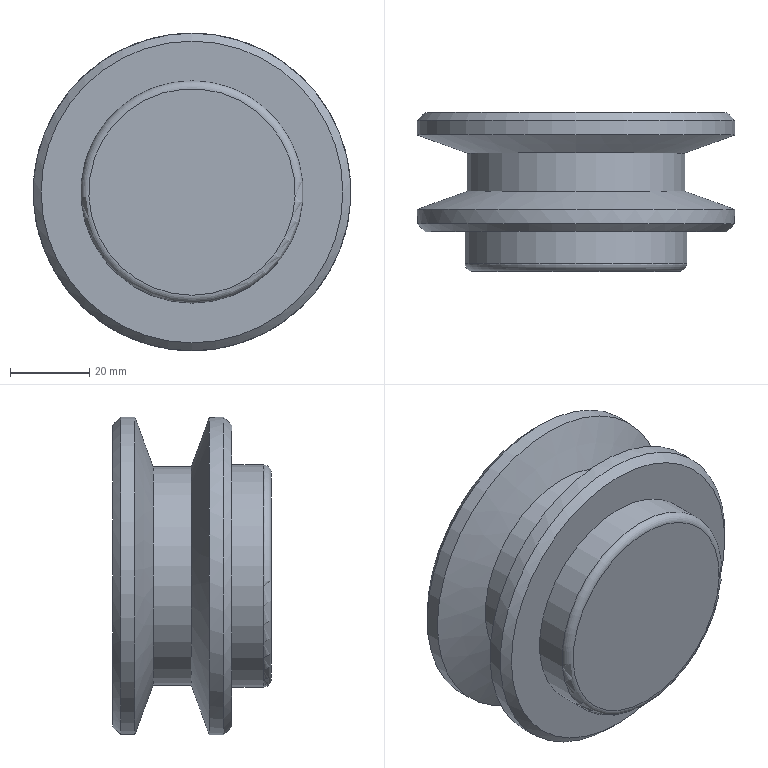Part | STEP file | Tube feed_id138_x_t | 1 solid | 12 faces | box 80 x 40 x 80 mm | volume 135943 mm3 | cylinder 4 | cone 4 | plane 3 | torus 1 | commonest cylinder face diameters 80 x2 55 x1 56 x1
STEP:
#1=CARTESIAN_POINT('',(0.,0.,0.));
#2=DIRECTION('',(0.,0.,1.));
#3=DIRECTION('',(1.,0.,0.));
#4=AXIS2_PLACEMENT_3D('',#1,#2,#3);
#5=CARTESIAN_POINT('',(-268.5,583.936,-125.5));
#6=VERTEX_POINT('',#5);
#7=CARTESIAN_POINT('',(-268.5,583.936,-205.5));
#8=VERTEX_POINT('',#7);
#9=CARTESIAN_POINT('',(-268.5,583.936,-165.5));
#10=DIRECTION('',(0.,1.,0.));
#11=DIRECTION('',(0.,0.,1.));
#12=AXIS2_PLACEMENT_3D('',#9,#10,#11);
#13=CIRCLE('',#12,40.);
#14=CARTESIAN_POINT('',(-268.5,601.936,-165.5));
#15=DIRECTION('',(0.,-1.,0.));
#16=DIRECTION('',(0.,0.,-1.));
#17=AXIS2_PLACEMENT_3D('',#14,#15,#16);
#18=CYLINDRICAL_SURFACE('',#17,40.);
#19=CARTESIAN_POINT('',(3.142,18.));
#20=DIRECTION('',(-1.,0.));
#21=VECTOR('',#20,1.);
#22=LINE('',#19,#21);
#23=(GEOMETRIC_REPRESENTATION_CONTEXT(2)PARAMETRIC_REPRESENTATION_CONTEXT()REPRESENTATION_CONTEXT('',''));
#24=DEFINITIONAL_REPRESENTATION('',(#22),#23);
#25=PCURVE('',#18,#24);
#26=CARTESIAN_POINT('',(-268.5,583.936,-165.5));
#27=DIRECTION('',(0.,1.,0.));
#28=DIRECTION('',(0.,0.,1.));
#29=AXIS2_PLACEMENT_3D('',#26,#27,#28);
#30=CONICAL_SURFACE('',#29,40.,0.7854);
#31=CARTESIAN_POINT('',(0.,0.));
#32=DIRECTION('',(1.,0.));
#33=VECTOR('',#32,1.);
#34=LINE('',#31,#33);
#35=(GEOMETRIC_REPRESENTATION_CONTEXT(2)PARAMETRIC_REPRESENTATION_CONTEXT()REPRESENTATION_CONTEXT('',''));
#36=DEFINITIONAL_REPRESENTATION('',(#34),#35);
#37=PCURVE('',#30,#36);
#38=SURFACE_CURVE('',#13,(#25,#37),.PCURVE_S1.);
#39=EDGE_CURVE('',#6,#8,#38,.T.);
#40=ORIENTED_EDGE('',*,*,#39,.T.);
#41=CARTESIAN_POINT('',(-268.5,587.568,-205.5));
#42=VERTEX_POINT('',#41);
#43=CARTESIAN_POINT('',(-268.5,587.568,-205.5));
#44=CARTESIAN_POINT('',(-268.5,583.936,-205.5));
#45=B_SPLINE_CURVE_WITH_KNOTS('',1,(#43,#44),.UNSPECIFIED.,.F.,.F.,(2,2),(14.368,18.),.PIECEWISE_BEZIER_KNOTS.);
#46=CARTESIAN_POINT('',(0.,0.));
#47=DIRECTION('',(0.,1.));
#48=VECTOR('',#47,1.);
#49=LINE('',#46,#48);
#50=(GEOMETRIC_REPRESENTATION_CONTEXT(2)PARAMETRIC_REPRESENTATION_CONTEXT()REPRESENTATION_CONTEXT('',''));
#51=DEFINITIONAL_REPRESENTATION('',(#49),#50);
#52=PCURVE('',#18,#51);
#53=CARTESIAN_POINT('',(6.283,0.));
#54=DIRECTION('',(0.,1.));
#55=VECTOR('',#54,1.);
#56=LINE('',#53,#55);
#57=(GEOMETRIC_REPRESENTATION_CONTEXT(2)PARAMETRIC_REPRESENTATION_CONTEXT()REPRESENTATION_CONTEXT('',''));
#58=DEFINITIONAL_REPRESENTATION('',(#56),#57);
#59=PCURVE('',#18,#58);
#60=SEAM_CURVE('',#45,(#52,#59),.PCURVE_S1.);
#61=EDGE_CURVE('',#42,#8,#60,.T.);
#62=ORIENTED_EDGE('',*,*,#61,.F.);
#63=CARTESIAN_POINT('',(-268.5,587.568,-165.5));
#64=DIRECTION('',(0.,1.,0.));
#65=DIRECTION('',(0.,0.,-1.));
#66=AXIS2_PLACEMENT_3D('',#63,#64,#65);
#67=CIRCLE('',#66,40.);
#68=CARTESIAN_POINT('',(6.283,14.368));
#69=DIRECTION('',(-1.,0.));
#70=VECTOR('',#69,1.);
#71=LINE('',#68,#70);
#72=(GEOMETRIC_REPRESENTATION_CONTEXT(2)PARAMETRIC_REPRESENTATION_CONTEXT()REPRESENTATION_CONTEXT('',''));
#73=DEFINITIONAL_REPRESENTATION('',(#71),#72);
#74=PCURVE('',#18,#73);
#75=CARTESIAN_POINT('',(-268.5,591.936,-165.5));
#76=DIRECTION('',(0.,-1.,0.));
#77=DIRECTION('',(0.,0.,-1.));
#78=AXIS2_PLACEMENT_3D('',#75,#76,#77);
#79=CONICAL_SURFACE('',#78,28.,1.222);
#80=CARTESIAN_POINT('',(6.283,4.368));
#81=DIRECTION('',(-1.,0.));
#82=VECTOR('',#81,1.);
#83=LINE('',#80,#82);
#84=(GEOMETRIC_REPRESENTATION_CONTEXT(2)PARAMETRIC_REPRESENTATION_CONTEXT()REPRESENTATION_CONTEXT('',''));
#85=DEFINITIONAL_REPRESENTATION('',(#83),#84);
#86=PCURVE('',#79,#85);
#87=SURFACE_CURVE('',#67,(#74,#86),.PCURVE_S1.);
#88=EDGE_CURVE('',#42,#42,#87,.T.);
#89=ORIENTED_EDGE('',*,*,#88,.F.);
#90=ORIENTED_EDGE('',*,*,#61,.T.);
#91=CARTESIAN_POINT('',(-268.5,583.936,-165.5));
#92=DIRECTION('',(0.,1.,0.));
#93=DIRECTION('',(0.,0.,1.));
#94=AXIS2_PLACEMENT_3D('',#91,#92,#93);
#95=CIRCLE('',#94,40.);
#96=CARTESIAN_POINT('',(9.425,18.));
#97=DIRECTION('',(-1.,0.));
#98=VECTOR('',#97,1.);
#99=LINE('',#96,#98);
#100=(GEOMETRIC_REPRESENTATION_CONTEXT(2)PARAMETRIC_REPRESENTATION_CONTEXT()REPRESENTATION_CONTEXT('',''));
#101=DEFINITIONAL_REPRESENTATION('',(#99),#100);
#102=PCURVE('',#18,#101);
#103=CARTESIAN_POINT('',(0.,0.));
#104=DIRECTION('',(1.,0.));
#105=VECTOR('',#104,1.);
#106=LINE('',#103,#105);
#107=(GEOMETRIC_REPRESENTATION_CONTEXT(2)PARAMETRIC_REPRESENTATION_CONTEXT()REPRESENTATION_CONTEXT('',''));
#108=DEFINITIONAL_REPRESENTATION('',(#106),#107);
#109=PCURVE('',#30,#108);
#110=SURFACE_CURVE('',#95,(#102,#109),.PCURVE_S1.);
#111=EDGE_CURVE('',#8,#6,#110,.T.);
#112=ORIENTED_EDGE('',*,*,#111,.T.);
#113=EDGE_LOOP('',(#40,#62,#89,#90,#112));
#114=FACE_BOUND('',#113,.T.);
#115=ADVANCED_FACE('',(#114),#18,.T.);
#116=CARTESIAN_POINT('',(-268.5,581.936,-193.5));
#117=VERTEX_POINT('',#116);
#118=CARTESIAN_POINT('',(-268.5,581.936,-165.5));
#119=DIRECTION('',(0.,-1.,0.));
#120=DIRECTION('',(0.,0.,-1.));
#121=AXIS2_PLACEMENT_3D('',#118,#119,#120);
#122=CIRCLE('',#121,28.);
#123=CARTESIAN_POINT('',(-268.5,581.936,-165.5));
#124=DIRECTION('',(0.,1.,0.));
#125=DIRECTION('',(0.,0.,1.));
#126=AXIS2_PLACEMENT_3D('',#123,#124,#125);
#127=PLANE('',#126);
#128=CARTESIAN_POINT('',(-28.,0.));
#129=CARTESIAN_POINT('',(-28.,48.497));
#130=CARTESIAN_POINT('',(14.,24.249));
#131=CARTESIAN_POINT('',(56.,0.));
#132=CARTESIAN_POINT('',(14.,-24.249));
#133=CARTESIAN_POINT('',(-28.,-48.497));
#134=CARTESIAN_POINT('',(-28.,0.));
#135=(BOUNDED_CURVE()B_SPLINE_CURVE(2,(#128,#129,#130,#131,#132,#133,#134),.UNSPECIFIED.,.T.,.F.)B_SPLINE_CURVE_WITH_KNOTS((1,2,2,2,2,1),(-2.094,0.,2.094,4.189,6.283,8.378),.UNSPECIFIED.)CURVE()GEOMETRIC_REPRESENTATION_ITEM()RATIONAL_B_SPLINE_CURVE((1.,0.5,1.,0.5,1.,0.5,1.))REPRESENTATION_ITEM(''));
#136=(GEOMETRIC_REPRESENTATION_CONTEXT(2)PARAMETRIC_REPRESENTATION_CONTEXT()REPRESENTATION_CONTEXT('',''));
#137=DEFINITIONAL_REPRESENTATION('',(#135),#136);
#138=PCURVE('',#127,#137);
#139=CARTESIAN_POINT('',(-268.5,571.936,-165.5));
#140=DIRECTION('',(0.,1.,0.));
#141=DIRECTION('',(0.,0.,1.));
#142=AXIS2_PLACEMENT_3D('',#139,#140,#141);
#143=CYLINDRICAL_SURFACE('',#142,28.);
#144=CARTESIAN_POINT('',(9.425,10.));
#145=DIRECTION('',(-1.,0.));
#146=VECTOR('',#145,1.);
#147=LINE('',#144,#146);
#148=(GEOMETRIC_REPRESENTATION_CONTEXT(2)PARAMETRIC_REPRESENTATION_CONTEXT()REPRESENTATION_CONTEXT('',''));
#149=DEFINITIONAL_REPRESENTATION('',(#147),#148);
#150=PCURVE('',#143,#149);
#151=SURFACE_CURVE('',#122,(#138,#150),.PCURVE_S1.);
#152=EDGE_CURVE('',#117,#117,#151,.T.);
#153=ORIENTED_EDGE('',*,*,#152,.F.);
#154=EDGE_LOOP('',(#153));
#155=FACE_BOUND('',#154,.T.);
#156=CARTESIAN_POINT('',(-268.5,581.936,-127.5));
#157=VERTEX_POINT('',#156);
#158=CARTESIAN_POINT('',(-268.5,581.936,-165.5));
#159=DIRECTION('',(0.,-1.,0.));
#160=DIRECTION('',(0.,0.,1.));
#161=AXIS2_PLACEMENT_3D('',#158,#159,#160);
#162=CIRCLE('',#161,38.);
#163=CARTESIAN_POINT('',(38.,0.));
#164=CARTESIAN_POINT('',(38.,-65.818));
#165=CARTESIAN_POINT('',(-19.,-32.909));
#166=CARTESIAN_POINT('',(-76.,0.));
#167=CARTESIAN_POINT('',(-19.,32.909));
#168=CARTESIAN_POINT('',(38.,65.818));
#169=CARTESIAN_POINT('',(38.,0.));
#170=(BOUNDED_CURVE()B_SPLINE_CURVE(2,(#163,#164,#165,#166,#167,#168,#169),.UNSPECIFIED.,.T.,.F.)B_SPLINE_CURVE_WITH_KNOTS((1,2,2,2,2,1),(-2.094,0.,2.094,4.189,6.283,8.378),.UNSPECIFIED.)CURVE()GEOMETRIC_REPRESENTATION_ITEM()RATIONAL_B_SPLINE_CURVE((1.,0.5,1.,0.5,1.,0.5,1.))REPRESENTATION_ITEM(''));
#171=(GEOMETRIC_REPRESENTATION_CONTEXT(2)PARAMETRIC_REPRESENTATION_CONTEXT()REPRESENTATION_CONTEXT('',''));
#172=DEFINITIONAL_REPRESENTATION('',(#170),#171);
#173=PCURVE('',#127,#172);
#174=CARTESIAN_POINT('',(6.283,-2.));
#175=DIRECTION('',(-1.,0.));
#176=VECTOR('',#175,1.);
#177=LINE('',#174,#176);
#178=(GEOMETRIC_REPRESENTATION_CONTEXT(2)PARAMETRIC_REPRESENTATION_CONTEXT()REPRESENTATION_CONTEXT('',''));
#179=DEFINITIONAL_REPRESENTATION('',(#177),#178);
#180=PCURVE('',#30,#179);
#181=SURFACE_CURVE('',#162,(#173,#180),.PCURVE_S1.);
#182=EDGE_CURVE('',#157,#157,#181,.T.);
#183=ORIENTED_EDGE('',*,*,#182,.T.);
#184=EDGE_LOOP('',(#183));
#185=FACE_BOUND('',#184,.T.);
#186=ADVANCED_FACE('',(#155,#185),#127,.F.);
#187=ORIENTED_EDGE('',*,*,#182,.F.);
#188=CARTESIAN_POINT('',(-268.5,581.936,-127.5));
#189=CARTESIAN_POINT('',(-268.5,583.936,-125.5));
#190=B_SPLINE_CURVE_WITH_KNOTS('',1,(#188,#189),.UNSPECIFIED.,.F.,.F.,(2,2),(-2.828,0.),.PIECEWISE_BEZIER_KNOTS.);
#191=CARTESIAN_POINT('',(6.283,0.));
#192=DIRECTION('',(0.,1.));
#193=VECTOR('',#192,1.);
#194=LINE('',#191,#193);
#195=(GEOMETRIC_REPRESENTATION_CONTEXT(2)PARAMETRIC_REPRESENTATION_CONTEXT()REPRESENTATION_CONTEXT('',''));
#196=DEFINITIONAL_REPRESENTATION('',(#194),#195);
#197=PCURVE('',#30,#196);
#198=CARTESIAN_POINT('',(0.,0.));
#199=DIRECTION('',(0.,1.));
#200=VECTOR('',#199,1.);
#201=LINE('',#198,#200);
#202=(GEOMETRIC_REPRESENTATION_CONTEXT(2)PARAMETRIC_REPRESENTATION_CONTEXT()REPRESENTATION_CONTEXT('',''));
#203=DEFINITIONAL_REPRESENTATION('',(#201),#202);
#204=PCURVE('',#30,#203);
#205=SEAM_CURVE('',#190,(#197,#204),.PCURVE_S1.);
#206=EDGE_CURVE('',#157,#6,#205,.T.);
#207=ORIENTED_EDGE('',*,*,#206,.T.);
#208=ORIENTED_EDGE('',*,*,#111,.F.);
#209=ORIENTED_EDGE('',*,*,#39,.F.);
#210=ORIENTED_EDGE('',*,*,#206,.F.);
#211=EDGE_LOOP('',(#187,#207,#208,#209,#210));
#212=FACE_BOUND('',#211,.T.);
#213=ADVANCED_FACE('',(#212),#30,.T.);
#214=CARTESIAN_POINT('',(-268.5,573.936,-193.5));
#215=VERTEX_POINT('',#214);
#216=CARTESIAN_POINT('',(-268.5,573.936,-165.5));
#217=DIRECTION('',(0.,1.,0.));
#218=DIRECTION('',(0.,0.,-1.));
#219=AXIS2_PLACEMENT_3D('',#216,#217,#218);
#220=CIRCLE('',#219,28.);
#221=CARTESIAN_POINT('',(3.142,2.));
#222=DIRECTION('',(1.,0.));
#223=VECTOR('',#222,1.);
#224=LINE('',#221,#223);
#225=(GEOMETRIC_REPRESENTATION_CONTEXT(2)PARAMETRIC_REPRESENTATION_CONTEXT()REPRESENTATION_CONTEXT('',''));
#226=DEFINITIONAL_REPRESENTATION('',(#224),#225);
#227=PCURVE('',#143,#226);
#228=CARTESIAN_POINT('',(-268.5,573.936,-165.5));
#229=DIRECTION('',(0.,-1.,0.));
#230=DIRECTION('',(0.,0.,-1.));
#231=AXIS2_PLACEMENT_3D('',#228,#229,#230);
#232=TOROIDAL_SURFACE('',#231,26.,2.);
#233=CARTESIAN_POINT('',(6.283,6.283));
#234=DIRECTION('',(-1.,0.));
#235=VECTOR('',#234,1.);
#236=LINE('',#233,#235);
#237=(GEOMETRIC_REPRESENTATION_CONTEXT(2)PARAMETRIC_REPRESENTATION_CONTEXT()REPRESENTATION_CONTEXT('',''));
#238=DEFINITIONAL_REPRESENTATION('',(#236),#237);
#239=PCURVE('',#232,#238);
#240=SURFACE_CURVE('',#220,(#227,#239),.PCURVE_S1.);
#241=EDGE_CURVE('',#215,#215,#240,.T.);
#242=ORIENTED_EDGE('',*,*,#241,.T.);
#243=CARTESIAN_POINT('',(-268.5,573.936,-193.5));
#244=CARTESIAN_POINT('',(-268.5,581.936,-193.5));
#245=B_SPLINE_CURVE_WITH_KNOTS('',1,(#243,#244),.UNSPECIFIED.,.F.,.F.,(2,2),(2.,10.),.PIECEWISE_BEZIER_KNOTS.);
#246=CARTESIAN_POINT('',(9.425,0.));
#247=DIRECTION('',(0.,1.));
#248=VECTOR('',#247,1.);
#249=LINE('',#246,#248);
#250=(GEOMETRIC_REPRESENTATION_CONTEXT(2)PARAMETRIC_REPRESENTATION_CONTEXT()REPRESENTATION_CONTEXT('',''));
#251=DEFINITIONAL_REPRESENTATION('',(#249),#250);
#252=PCURVE('',#143,#251);
#253=CARTESIAN_POINT('',(3.142,0.));
#254=DIRECTION('',(0.,1.));
#255=VECTOR('',#254,1.);
#256=LINE('',#253,#255);
#257=(GEOMETRIC_REPRESENTATION_CONTEXT(2)PARAMETRIC_REPRESENTATION_CONTEXT()REPRESENTATION_CONTEXT('',''));
#258=DEFINITIONAL_REPRESENTATION('',(#256),#257);
#259=PCURVE('',#143,#258);
#260=SEAM_CURVE('',#245,(#252,#259),.PCURVE_S1.);
#261=EDGE_CURVE('',#215,#117,#260,.T.);
#262=ORIENTED_EDGE('',*,*,#261,.T.);
#263=ORIENTED_EDGE('',*,*,#152,.T.);
#264=ORIENTED_EDGE('',*,*,#261,.F.);
#265=EDGE_LOOP('',(#242,#262,#263,#264));
#266=FACE_BOUND('',#265,.T.);
#267=ADVANCED_FACE('',(#266),#143,.T.);
#268=CARTESIAN_POINT('',(-268.5,571.936,-191.5));
#269=VERTEX_POINT('',#268);
#270=CARTESIAN_POINT('',(-268.5,571.936,-165.5));
#271=DIRECTION('',(0.,-1.,0.));
#272=DIRECTION('',(0.,0.,-1.));
#273=AXIS2_PLACEMENT_3D('',#270,#271,#272);
#274=CIRCLE('',#273,26.);
#275=CARTESIAN_POINT('',(-268.5,571.936,-165.5));
#276=DIRECTION('',(0.,-1.,0.));
#277=DIRECTION('',(0.,0.,-1.));
#278=AXIS2_PLACEMENT_3D('',#275,#276,#277);
#279=PLANE('',#278);
#280=CARTESIAN_POINT('',(0.,0.));
#281=DIRECTION('',(1.,0.));
#282=AXIS2_PLACEMENT_2D('',#280,#281);
#283=CIRCLE('',#282,26.);
#284=(GEOMETRIC_REPRESENTATION_CONTEXT(2)PARAMETRIC_REPRESENTATION_CONTEXT()REPRESENTATION_CONTEXT('',''));
#285=DEFINITIONAL_REPRESENTATION('',(#283),#284);
#286=PCURVE('',#279,#285);
#287=CARTESIAN_POINT('',(0.,7.854));
#288=DIRECTION('',(1.,0.));
#289=VECTOR('',#288,1.);
#290=LINE('',#287,#289);
#291=(GEOMETRIC_REPRESENTATION_CONTEXT(2)PARAMETRIC_REPRESENTATION_CONTEXT()REPRESENTATION_CONTEXT('',''));
#292=DEFINITIONAL_REPRESENTATION('',(#290),#291);
#293=PCURVE('',#232,#292);
#294=SURFACE_CURVE('',#274,(#286,#293),.PCURVE_S1.);
#295=EDGE_CURVE('',#269,#269,#294,.T.);
#296=ORIENTED_EDGE('',*,*,#295,.T.);
#297=EDGE_LOOP('',(#296));
#298=FACE_BOUND('',#297,.T.);
#299=ADVANCED_FACE('',(#298),#279,.T.);
#300=ORIENTED_EDGE('',*,*,#241,.F.);
#301=CARTESIAN_POINT('',(-268.5,573.936,-193.5));
#302=CARTESIAN_POINT('',(-268.5,573.401,-193.5));
#303=CARTESIAN_POINT('',(-268.5,572.88,-193.33));
#304=CARTESIAN_POINT('',(-268.5,572.432,-193.004));
#305=CARTESIAN_POINT('',(-268.5,572.106,-192.555));
#306=CARTESIAN_POINT('',(-268.5,571.936,-192.035));
#307=CARTESIAN_POINT('',(-268.5,571.936,-191.5));
#308=(BOUNDED_CURVE()B_SPLINE_CURVE(6,(#301,#302,#303,#304,#305,#306,#307),.UNSPECIFIED.,.F.,.F.)B_SPLINE_CURVE_WITH_KNOTS((7,7),(0.,1.571),.PIECEWISE_BEZIER_KNOTS.)CURVE()GEOMETRIC_REPRESENTATION_ITEM()RATIONAL_B_SPLINE_CURVE((1.031,1.01,0.9979,0.994,0.9979,1.01,1.031))REPRESENTATION_ITEM(''));
#309=CARTESIAN_POINT('',(6.283,6.283));
#310=DIRECTION('',(0.,1.));
#311=VECTOR('',#310,1.);
#312=LINE('',#309,#311);
#313=(GEOMETRIC_REPRESENTATION_CONTEXT(2)PARAMETRIC_REPRESENTATION_CONTEXT()REPRESENTATION_CONTEXT('',''));
#314=DEFINITIONAL_REPRESENTATION('',(#312),#313);
#315=PCURVE('',#232,#314);
#316=CARTESIAN_POINT('',(0.,6.283));
#317=DIRECTION('',(0.,1.));
#318=VECTOR('',#317,1.);
#319=LINE('',#316,#318);
#320=(GEOMETRIC_REPRESENTATION_CONTEXT(2)PARAMETRIC_REPRESENTATION_CONTEXT()REPRESENTATION_CONTEXT('',''));
#321=DEFINITIONAL_REPRESENTATION('',(#319),#320);
#322=PCURVE('',#232,#321);
#323=SEAM_CURVE('',#308,(#315,#322),.PCURVE_S1.);
#324=EDGE_CURVE('',#215,#269,#323,.T.);
#325=ORIENTED_EDGE('',*,*,#324,.T.);
#326=ORIENTED_EDGE('',*,*,#295,.F.);
#327=ORIENTED_EDGE('',*,*,#324,.F.);
#328=EDGE_LOOP('',(#300,#325,#326,#327));
#329=FACE_BOUND('',#328,.T.);
#330=ADVANCED_FACE('',(#329),#232,.T.);
#331=CARTESIAN_POINT('',(-268.5,592.118,-193.));
#332=VERTEX_POINT('',#331);
#333=CARTESIAN_POINT('',(-268.5,592.118,-138.));
#334=VERTEX_POINT('',#333);
#335=CARTESIAN_POINT('',(-268.5,592.118,-165.5));
#336=DIRECTION('',(0.,-1.,0.));
#337=DIRECTION('',(0.,0.,-1.));
#338=AXIS2_PLACEMENT_3D('',#335,#336,#337);
#339=CIRCLE('',#338,27.5);
#340=CARTESIAN_POINT('',(0.,-0.182));
#341=DIRECTION('',(1.,0.));
#342=VECTOR('',#341,1.);
#343=LINE('',#340,#342);
#344=(GEOMETRIC_REPRESENTATION_CONTEXT(2)PARAMETRIC_REPRESENTATION_CONTEXT()REPRESENTATION_CONTEXT('',''));
#345=DEFINITIONAL_REPRESENTATION('',(#343),#344);
#346=PCURVE('',#79,#345);
#347=CARTESIAN_POINT('',(-268.5,601.936,-165.5));
#348=DIRECTION('',(0.,1.,0.));
#349=DIRECTION('',(0.,0.,1.));
#350=AXIS2_PLACEMENT_3D('',#347,#348,#349);
#351=CYLINDRICAL_SURFACE('',#350,27.5);
#352=CARTESIAN_POINT('',(3.142,-9.818));
#353=DIRECTION('',(-1.,0.));
#354=VECTOR('',#353,1.);
#355=LINE('',#352,#354);
#356=(GEOMETRIC_REPRESENTATION_CONTEXT(2)PARAMETRIC_REPRESENTATION_CONTEXT()REPRESENTATION_CONTEXT('',''));
#357=DEFINITIONAL_REPRESENTATION('',(#355),#356);
#358=PCURVE('',#351,#357);
#359=SURFACE_CURVE('',#339,(#346,#358),.PCURVE_S1.);
#360=EDGE_CURVE('',#332,#334,#359,.T.);
#361=ORIENTED_EDGE('',*,*,#360,.T.);
#362=CARTESIAN_POINT('',(-268.5,592.118,-165.5));
#363=DIRECTION('',(0.,-1.,0.));
#364=DIRECTION('',(0.,0.,-1.));
#365=AXIS2_PLACEMENT_3D('',#362,#363,#364);
#366=CIRCLE('',#365,27.5);
#367=CARTESIAN_POINT('',(0.,-0.182));
#368=DIRECTION('',(1.,0.));
#369=VECTOR('',#368,1.);
#370=LINE('',#367,#369);
#371=(GEOMETRIC_REPRESENTATION_CONTEXT(2)PARAMETRIC_REPRESENTATION_CONTEXT()REPRESENTATION_CONTEXT('',''));
#372=DEFINITIONAL_REPRESENTATION('',(#370),#371);
#373=PCURVE('',#79,#372);
#374=CARTESIAN_POINT('',(9.425,-9.818));
#375=DIRECTION('',(-1.,0.));
#376=VECTOR('',#375,1.);
#377=LINE('',#374,#376);
#378=(GEOMETRIC_REPRESENTATION_CONTEXT(2)PARAMETRIC_REPRESENTATION_CONTEXT()REPRESENTATION_CONTEXT('',''));
#379=DEFINITIONAL_REPRESENTATION('',(#377),#378);
#380=PCURVE('',#351,#379);
#381=SURFACE_CURVE('',#366,(#373,#380),.PCURVE_S1.);
#382=EDGE_CURVE('',#334,#332,#381,.T.);
#383=ORIENTED_EDGE('',*,*,#382,.T.);
#384=CARTESIAN_POINT('',(-268.5,592.118,-193.));
#385=CARTESIAN_POINT('',(-268.5,587.568,-205.5));
#386=B_SPLINE_CURVE_WITH_KNOTS('',1,(#384,#385),.UNSPECIFIED.,.F.,.F.,(2,2),(-0.5321,12.77),.PIECEWISE_BEZIER_KNOTS.);
#387=CARTESIAN_POINT('',(6.283,0.));
#388=DIRECTION('',(0.,1.));
#389=VECTOR('',#388,1.);
#390=LINE('',#387,#389);
#391=(GEOMETRIC_REPRESENTATION_CONTEXT(2)PARAMETRIC_REPRESENTATION_CONTEXT()REPRESENTATION_CONTEXT('',''));
#392=DEFINITIONAL_REPRESENTATION('',(#390),#391);
#393=PCURVE('',#79,#392);
#394=CARTESIAN_POINT('',(0.,0.));
#395=DIRECTION('',(0.,1.));
#396=VECTOR('',#395,1.);
#397=LINE('',#394,#396);
#398=(GEOMETRIC_REPRESENTATION_CONTEXT(2)PARAMETRIC_REPRESENTATION_CONTEXT()REPRESENTATION_CONTEXT('',''));
#399=DEFINITIONAL_REPRESENTATION('',(#397),#398);
#400=PCURVE('',#79,#399);
#401=SEAM_CURVE('',#386,(#393,#400),.PCURVE_S1.);
#402=EDGE_CURVE('',#332,#42,#401,.T.);
#403=ORIENTED_EDGE('',*,*,#402,.T.);
#404=ORIENTED_EDGE('',*,*,#88,.T.);
#405=ORIENTED_EDGE('',*,*,#402,.F.);
#406=EDGE_LOOP('',(#361,#383,#403,#404,#405));
#407=FACE_BOUND('',#406,.T.);
#408=ADVANCED_FACE('',(#407),#79,.T.);
#409=CARTESIAN_POINT('',(-268.5,601.754,-138.));
#410=VERTEX_POINT('',#409);
#411=CARTESIAN_POINT('',(-268.5,601.754,-165.5));
#412=DIRECTION('',(0.,-1.,0.));
#413=DIRECTION('',(0.,0.,1.));
#414=AXIS2_PLACEMENT_3D('',#411,#412,#413);
#415=CIRCLE('',#414,27.5);
#416=CARTESIAN_POINT('',(-268.5,606.689,-165.5));
#417=DIRECTION('',(0.,1.,0.));
#418=DIRECTION('',(0.,0.,1.));
#419=AXIS2_PLACEMENT_3D('',#416,#417,#418);
#420=CONICAL_SURFACE('',#419,41.06,1.222);
#421=CARTESIAN_POINT('',(6.283,-4.936));
#422=DIRECTION('',(-1.,0.));
#423=VECTOR('',#422,1.);
#424=LINE('',#421,#423);
#425=(GEOMETRIC_REPRESENTATION_CONTEXT(2)PARAMETRIC_REPRESENTATION_CONTEXT()REPRESENTATION_CONTEXT('',''));
#426=DEFINITIONAL_REPRESENTATION('',(#424),#425);
#427=PCURVE('',#420,#426);
#428=CARTESIAN_POINT('',(6.283,-0.182));
#429=DIRECTION('',(-1.,0.));
#430=VECTOR('',#429,1.);
#431=LINE('',#428,#430);
#432=(GEOMETRIC_REPRESENTATION_CONTEXT(2)PARAMETRIC_REPRESENTATION_CONTEXT()REPRESENTATION_CONTEXT('',''));
#433=DEFINITIONAL_REPRESENTATION('',(#431),#432);
#434=PCURVE('',#351,#433);
#435=SURFACE_CURVE('',#415,(#427,#434),.PCURVE_S1.);
#436=EDGE_CURVE('',#410,#410,#435,.T.);
#437=ORIENTED_EDGE('',*,*,#436,.F.);
#438=CARTESIAN_POINT('',(-268.5,606.303,-125.5));
#439=VERTEX_POINT('',#438);
#440=CARTESIAN_POINT('',(-268.5,601.754,-138.));
#441=CARTESIAN_POINT('',(-268.5,606.303,-125.5));
#442=B_SPLINE_CURVE_WITH_KNOTS('',1,(#440,#441),.UNSPECIFIED.,.F.,.F.,(2,2),(-14.431,-1.128),.PIECEWISE_BEZIER_KNOTS.);
#443=CARTESIAN_POINT('',(6.283,0.));
#444=DIRECTION('',(0.,1.));
#445=VECTOR('',#444,1.);
#446=LINE('',#443,#445);
#447=(GEOMETRIC_REPRESENTATION_CONTEXT(2)PARAMETRIC_REPRESENTATION_CONTEXT()REPRESENTATION_CONTEXT('',''));
#448=DEFINITIONAL_REPRESENTATION('',(#446),#447);
#449=PCURVE('',#420,#448);
#450=CARTESIAN_POINT('',(0.,0.));
#451=DIRECTION('',(0.,1.));
#452=VECTOR('',#451,1.);
#453=LINE('',#450,#452);
#454=(GEOMETRIC_REPRESENTATION_CONTEXT(2)PARAMETRIC_REPRESENTATION_CONTEXT()REPRESENTATION_CONTEXT('',''));
#455=DEFINITIONAL_REPRESENTATION('',(#453),#454);
#456=PCURVE('',#420,#455);
#457=SEAM_CURVE('',#442,(#449,#456),.PCURVE_S1.);
#458=EDGE_CURVE('',#410,#439,#457,.T.);
#459=ORIENTED_EDGE('',*,*,#458,.T.);
#460=CARTESIAN_POINT('',(-268.5,606.303,-165.5));
#461=DIRECTION('',(0.,-1.,0.));
#462=DIRECTION('',(0.,0.,1.));
#463=AXIS2_PLACEMENT_3D('',#460,#461,#462);
#464=CIRCLE('',#463,40.);
#465=CARTESIAN_POINT('',(6.283,-0.3859));
#466=DIRECTION('',(-1.,0.));
#467=VECTOR('',#466,1.);
#468=LINE('',#465,#467);
#469=(GEOMETRIC_REPRESENTATION_CONTEXT(2)PARAMETRIC_REPRESENTATION_CONTEXT()REPRESENTATION_CONTEXT('',''));
#470=DEFINITIONAL_REPRESENTATION('',(#468),#469);
#471=PCURVE('',#420,#470);
#472=CARTESIAN_POINT('',(-268.5,601.936,-165.5));
#473=DIRECTION('',(0.,-1.,0.));
#474=DIRECTION('',(0.,0.,-1.));
#475=AXIS2_PLACEMENT_3D('',#472,#473,#474);
#476=CYLINDRICAL_SURFACE('',#475,40.);
#477=CARTESIAN_POINT('',(3.142,-4.368));
#478=DIRECTION('',(1.,0.));
#479=VECTOR('',#478,1.);
#480=LINE('',#477,#479);
#481=(GEOMETRIC_REPRESENTATION_CONTEXT(2)PARAMETRIC_REPRESENTATION_CONTEXT()REPRESENTATION_CONTEXT('',''));
#482=DEFINITIONAL_REPRESENTATION('',(#480),#481);
#483=PCURVE('',#476,#482);
#484=SURFACE_CURVE('',#464,(#471,#483),.PCURVE_S1.);
#485=EDGE_CURVE('',#439,#439,#484,.T.);
#486=ORIENTED_EDGE('',*,*,#485,.T.);
#487=ORIENTED_EDGE('',*,*,#458,.F.);
#488=EDGE_LOOP('',(#437,#459,#486,#487));
#489=FACE_BOUND('',#488,.T.);
#490=ADVANCED_FACE('',(#489),#420,.T.);
#491=ORIENTED_EDGE('',*,*,#382,.F.);
#492=CARTESIAN_POINT('',(-268.5,592.118,-138.));
#493=CARTESIAN_POINT('',(-268.5,601.754,-138.));
#494=B_SPLINE_CURVE_WITH_KNOTS('',1,(#492,#493),.UNSPECIFIED.,.F.,.F.,(2,2),(-9.818,-0.182),.PIECEWISE_BEZIER_KNOTS.);
#495=CARTESIAN_POINT('',(6.283,0.));
#496=DIRECTION('',(0.,1.));
#497=VECTOR('',#496,1.);
#498=LINE('',#495,#497);
#499=(GEOMETRIC_REPRESENTATION_CONTEXT(2)PARAMETRIC_REPRESENTATION_CONTEXT()REPRESENTATION_CONTEXT('',''));
#500=DEFINITIONAL_REPRESENTATION('',(#498),#499);
#501=PCURVE('',#351,#500);
#502=CARTESIAN_POINT('',(0.,0.));
#503=DIRECTION('',(0.,1.));
#504=VECTOR('',#503,1.);
#505=LINE('',#502,#504);
#506=(GEOMETRIC_REPRESENTATION_CONTEXT(2)PARAMETRIC_REPRESENTATION_CONTEXT()REPRESENTATION_CONTEXT('',''));
#507=DEFINITIONAL_REPRESENTATION('',(#505),#506);
#508=PCURVE('',#351,#507);
#509=SEAM_CURVE('',#494,(#501,#508),.PCURVE_S1.);
#510=EDGE_CURVE('',#334,#410,#509,.T.);
#511=ORIENTED_EDGE('',*,*,#510,.T.);
#512=ORIENTED_EDGE('',*,*,#436,.T.);
#513=ORIENTED_EDGE('',*,*,#510,.F.);
#514=ORIENTED_EDGE('',*,*,#360,.F.);
#515=EDGE_LOOP('',(#491,#511,#512,#513,#514));
#516=FACE_BOUND('',#515,.T.);
#517=ADVANCED_FACE('',(#516),#351,.T.);
#518=CARTESIAN_POINT('',(-268.5,611.936,-127.5));
#519=VERTEX_POINT('',#518);
#520=CARTESIAN_POINT('',(-268.5,611.936,-165.5));
#521=DIRECTION('',(0.,1.,0.));
#522=DIRECTION('',(0.,0.,1.));
#523=AXIS2_PLACEMENT_3D('',#520,#521,#522);
#524=CIRCLE('',#523,38.);
#525=CARTESIAN_POINT('',(-268.5,611.936,-165.5));
#526=DIRECTION('',(0.,1.,0.));
#527=DIRECTION('',(0.,0.,1.));
#528=AXIS2_PLACEMENT_3D('',#525,#526,#527);
#529=PLANE('',#528);
#530=CARTESIAN_POINT('',(0.,0.));
#531=DIRECTION('',(1.,0.));
#532=AXIS2_PLACEMENT_2D('',#530,#531);
#533=CIRCLE('',#532,38.);
#534=(GEOMETRIC_REPRESENTATION_CONTEXT(2)PARAMETRIC_REPRESENTATION_CONTEXT()REPRESENTATION_CONTEXT('',''));
#535=DEFINITIONAL_REPRESENTATION('',(#533),#534);
#536=PCURVE('',#529,#535);
#537=CARTESIAN_POINT('',(-268.5,611.936,-165.5));
#538=DIRECTION('',(0.,-1.,0.));
#539=DIRECTION('',(0.,0.,-1.));
#540=AXIS2_PLACEMENT_3D('',#537,#538,#539);
#541=CONICAL_SURFACE('',#540,38.,0.7854);
#542=CARTESIAN_POINT('',(9.425,0.));
#543=DIRECTION('',(-1.,0.));
#544=VECTOR('',#543,1.);
#545=LINE('',#542,#544);
#546=(GEOMETRIC_REPRESENTATION_CONTEXT(2)PARAMETRIC_REPRESENTATION_CONTEXT()REPRESENTATION_CONTEXT('',''));
#547=DEFINITIONAL_REPRESENTATION('',(#545),#546);
#548=PCURVE('',#541,#547);
#549=SURFACE_CURVE('',#524,(#536,#548),.PCURVE_S1.);
#550=EDGE_CURVE('',#519,#519,#549,.T.);
#551=ORIENTED_EDGE('',*,*,#550,.T.);
#552=EDGE_LOOP('',(#551));
#553=FACE_BOUND('',#552,.T.);
#554=ADVANCED_FACE('',(#553),#529,.T.);
#555=CARTESIAN_POINT('',(-268.5,609.936,-125.5));
#556=VERTEX_POINT('',#555);
#557=CARTESIAN_POINT('',(-268.5,609.936,-165.5));
#558=DIRECTION('',(0.,-1.,0.));
#559=DIRECTION('',(0.,0.,1.));
#560=AXIS2_PLACEMENT_3D('',#557,#558,#559);
#561=CIRCLE('',#560,40.);
#562=CARTESIAN_POINT('',(3.142,2.));
#563=DIRECTION('',(1.,0.));
#564=VECTOR('',#563,1.);
#565=LINE('',#562,#564);
#566=(GEOMETRIC_REPRESENTATION_CONTEXT(2)PARAMETRIC_REPRESENTATION_CONTEXT()REPRESENTATION_CONTEXT('',''));
#567=DEFINITIONAL_REPRESENTATION('',(#565),#566);
#568=PCURVE('',#541,#567);
#569=CARTESIAN_POINT('',(3.142,-8.));
#570=DIRECTION('',(1.,0.));
#571=VECTOR('',#570,1.);
#572=LINE('',#569,#571);
#573=(GEOMETRIC_REPRESENTATION_CONTEXT(2)PARAMETRIC_REPRESENTATION_CONTEXT()REPRESENTATION_CONTEXT('',''));
#574=DEFINITIONAL_REPRESENTATION('',(#572),#573);
#575=PCURVE('',#476,#574);
#576=SURFACE_CURVE('',#561,(#568,#575),.PCURVE_S1.);
#577=EDGE_CURVE('',#556,#556,#576,.T.);
#578=ORIENTED_EDGE('',*,*,#577,.F.);
#579=CARTESIAN_POINT('',(-268.5,611.936,-127.5));
#580=CARTESIAN_POINT('',(-268.5,609.936,-125.5));
#581=B_SPLINE_CURVE_WITH_KNOTS('',1,(#579,#580),.UNSPECIFIED.,.F.,.F.,(2,2),(0.,2.828),.PIECEWISE_BEZIER_KNOTS.);
#582=CARTESIAN_POINT('',(3.142,0.));
#583=DIRECTION('',(0.,1.));
#584=VECTOR('',#583,1.);
#585=LINE('',#582,#584);
#586=(GEOMETRIC_REPRESENTATION_CONTEXT(2)PARAMETRIC_REPRESENTATION_CONTEXT()REPRESENTATION_CONTEXT('',''));
#587=DEFINITIONAL_REPRESENTATION('',(#585),#586);
#588=PCURVE('',#541,#587);
#589=CARTESIAN_POINT('',(9.425,0.));
#590=DIRECTION('',(0.,1.));
#591=VECTOR('',#590,1.);
#592=LINE('',#589,#591);
#593=(GEOMETRIC_REPRESENTATION_CONTEXT(2)PARAMETRIC_REPRESENTATION_CONTEXT()REPRESENTATION_CONTEXT('',''));
#594=DEFINITIONAL_REPRESENTATION('',(#592),#593);
#595=PCURVE('',#541,#594);
#596=SEAM_CURVE('',#581,(#588,#595),.PCURVE_S1.);
#597=EDGE_CURVE('',#519,#556,#596,.T.);
#598=ORIENTED_EDGE('',*,*,#597,.F.);
#599=ORIENTED_EDGE('',*,*,#550,.F.);
#600=ORIENTED_EDGE('',*,*,#597,.T.);
#601=EDGE_LOOP('',(#578,#598,#599,#600));
#602=FACE_BOUND('',#601,.T.);
#603=ADVANCED_FACE('',(#602),#541,.T.);
#604=ORIENTED_EDGE('',*,*,#577,.T.);
#605=CARTESIAN_POINT('',(-268.5,609.936,-125.5));
#606=CARTESIAN_POINT('',(-268.5,606.303,-125.5));
#607=B_SPLINE_CURVE_WITH_KNOTS('',1,(#605,#606),.UNSPECIFIED.,.F.,.F.,(2,2),(-8.,-4.368),.PIECEWISE_BEZIER_KNOTS.);
#608=CARTESIAN_POINT('',(9.425,0.));
#609=DIRECTION('',(0.,1.));
#610=VECTOR('',#609,1.);
#611=LINE('',#608,#610);
#612=(GEOMETRIC_REPRESENTATION_CONTEXT(2)PARAMETRIC_REPRESENTATION_CONTEXT()REPRESENTATION_CONTEXT('',''));
#613=DEFINITIONAL_REPRESENTATION('',(#611),#612);
#614=PCURVE('',#476,#613);
#615=CARTESIAN_POINT('',(3.142,0.));
#616=DIRECTION('',(0.,1.));
#617=VECTOR('',#616,1.);
#618=LINE('',#615,#617);
#619=(GEOMETRIC_REPRESENTATION_CONTEXT(2)PARAMETRIC_REPRESENTATION_CONTEXT()REPRESENTATION_CONTEXT('',''));
#620=DEFINITIONAL_REPRESENTATION('',(#618),#619);
#621=PCURVE('',#476,#620);
#622=SEAM_CURVE('',#607,(#614,#621),.PCURVE_S1.);
#623=EDGE_CURVE('',#556,#439,#622,.T.);
#624=ORIENTED_EDGE('',*,*,#623,.T.);
#625=ORIENTED_EDGE('',*,*,#485,.F.);
#626=ORIENTED_EDGE('',*,*,#623,.F.);
#627=EDGE_LOOP('',(#604,#624,#625,#626));
#628=FACE_BOUND('',#627,.T.);
#629=ADVANCED_FACE('',(#628),#476,.T.);
#630=CLOSED_SHELL('',(#115,#186,#213,#267,#299,#330,#408,#490,#517,#554,#603,#629));
#631=MANIFOLD_SOLID_BREP('',#630);
#632=(LENGTH_UNIT()NAMED_UNIT(*)SI_UNIT(.MILLI.,.METRE.));
#633=UNCERTAINTY_MEASURE_WITH_UNIT(LENGTH_MEASURE(0.00001),#632,'','');
#634=(NAMED_UNIT(*)PLANE_ANGLE_UNIT()SI_UNIT($,.RADIAN.));
#635=(NAMED_UNIT(*)SI_UNIT($,.STERADIAN.)SOLID_ANGLE_UNIT());
#636=(GEOMETRIC_REPRESENTATION_CONTEXT(3)GLOBAL_UNCERTAINTY_ASSIGNED_CONTEXT((#633))GLOBAL_UNIT_ASSIGNED_CONTEXT((#632,#634,#635))REPRESENTATION_CONTEXT('',''));
#637=ADVANCED_BREP_SHAPE_REPRESENTATION('',(#4,#631),#636);